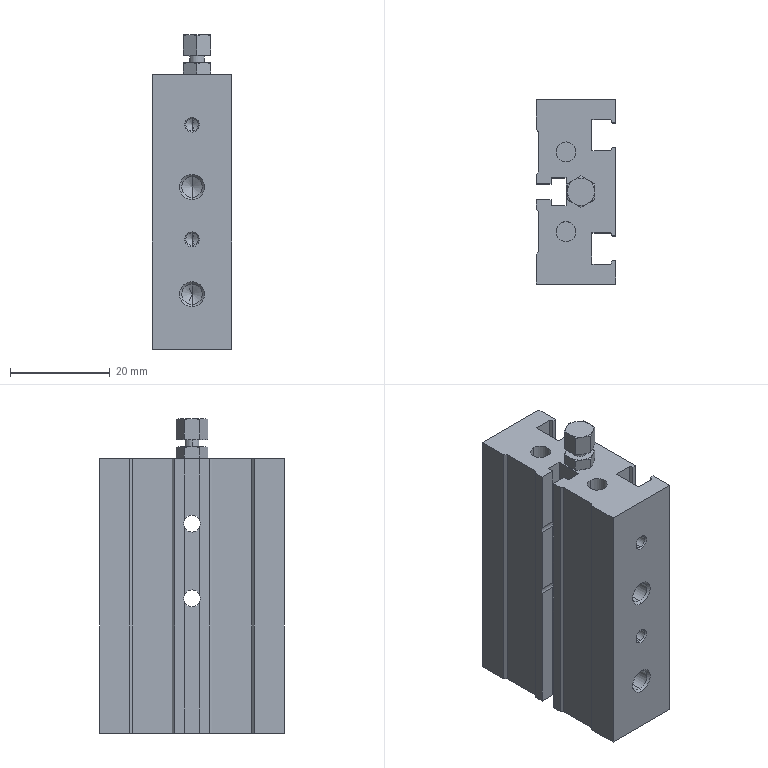Part | SolidWorks | features HoleWzd 12, RefAxis 9, 3DProfileFeature 3, RevCut 2, Revolution 2, Extrusion 1, ICE 1 | 1 solid | 169 faces | box 16 x 37 x 63 mm | volume 25617 mm3 | cone 64 | plane 63 | cylinder 42 | commonest cylinder face diameters 4.134 x12 2.459 x8 3.4 x8 4 x4 6 x4 6.5 x4